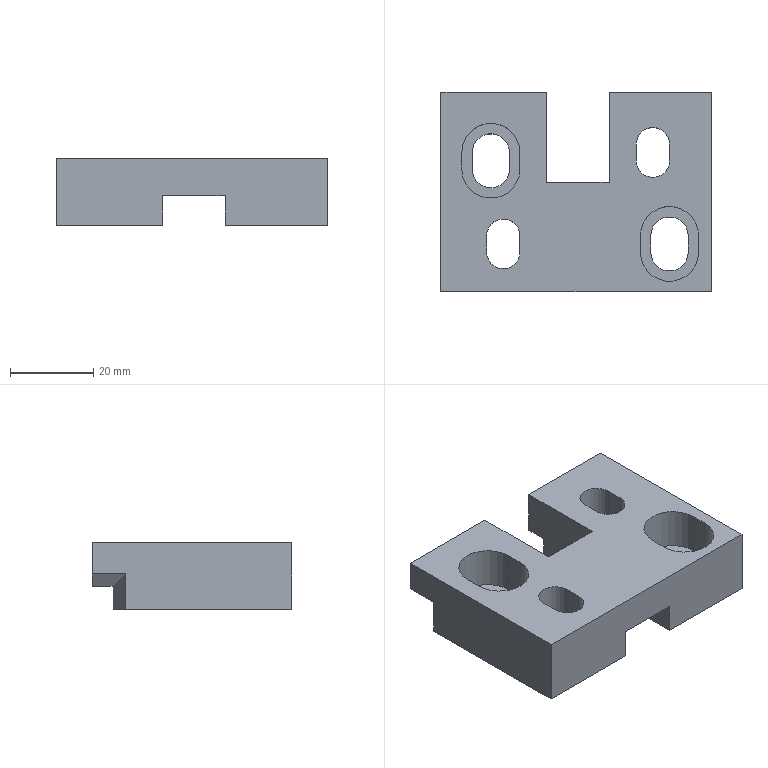Part | STEP file | 1 solid | 46 faces | box 65 x 48 x 16 mm | volume 32002 mm3 | plane 33 | cylinder 13 | commonest cylinder face diameters 8 x4 9 x4 14 x4 5 x1
STEP:
#1=CARTESIAN_POINT('',(-142.451,-110.8,-2.));
#2=VERTEX_POINT('',#1);
#3=CARTESIAN_POINT('',(-142.451,-110.8,4.));
#4=VERTEX_POINT('',#3);
#5=CARTESIAN_POINT('',(-142.451,-110.8,-2.));
#6=DIRECTION('',(0.,0.,1.));
#7=VECTOR('',#6,1.);
#8=LINE('',#5,#7);
#9=EDGE_CURVE('',#2,#4,#8,.T.);
#10=ORIENTED_EDGE('',*,*,#9,.T.);
#11=CARTESIAN_POINT('',(-151.451,-110.8,4.));
#12=VERTEX_POINT('',#11);
#13=CARTESIAN_POINT('',(-146.951,-110.8,4.));
#14=DIRECTION('',(0.,0.,-1.));
#15=DIRECTION('',(-1.,0.,0.));
#16=AXIS2_PLACEMENT_3D('',#13,#14,#15);
#17=CIRCLE('',#16,4.5);
#18=EDGE_CURVE('',#12,#4,#17,.T.);
#19=ORIENTED_EDGE('',*,*,#18,.F.);
#20=CARTESIAN_POINT('',(-151.451,-110.8,-2.));
#21=VERTEX_POINT('',#20);
#22=CARTESIAN_POINT('',(-151.451,-110.8,-2.));
#23=DIRECTION('',(0.,0.,1.));
#24=VECTOR('',#23,1.);
#25=LINE('',#22,#24);
#26=EDGE_CURVE('',#21,#12,#25,.T.);
#27=ORIENTED_EDGE('',*,*,#26,.F.);
#28=CARTESIAN_POINT('',(-146.951,-110.8,-2.));
#29=DIRECTION('',(0.,0.,-1.));
#30=DIRECTION('',(-1.,0.,0.));
#31=AXIS2_PLACEMENT_3D('',#28,#29,#30);
#32=CIRCLE('',#31,4.5);
#33=EDGE_CURVE('',#21,#2,#32,.T.);
#34=ORIENTED_EDGE('',*,*,#33,.T.);
#35=EDGE_LOOP('',(#10,#19,#27,#34));
#36=FACE_OUTER_BOUND('',#35,.T.);
#37=CARTESIAN_POINT('',(-146.951,-110.8,-2.));
#38=DIRECTION('',(0.,0.,1.));
#39=DIRECTION('',(1.,0.,0.));
#40=AXIS2_PLACEMENT_3D('',#37,#38,#39);
#41=CYLINDRICAL_SURFACE('',#40,4.5);
#42=ADVANCED_FACE('',(#36),#41,.F.);
#43=ORIENTED_EDGE('',*,*,#26,.T.);
#44=CARTESIAN_POINT('',(-151.451,-114.8,4.));
#45=VERTEX_POINT('',#44);
#46=CARTESIAN_POINT('',(-151.451,-116.3,4.));
#47=DIRECTION('',(0.,1.,0.));
#48=VECTOR('',#47,1.);
#49=LINE('',#46,#48);
#50=EDGE_CURVE('',#45,#12,#49,.T.);
#51=ORIENTED_EDGE('',*,*,#50,.F.);
#52=CARTESIAN_POINT('',(-151.451,-114.8,-2.));
#53=VERTEX_POINT('',#52);
#54=CARTESIAN_POINT('',(-151.451,-114.8,-2.));
#55=DIRECTION('',(0.,0.,1.));
#56=VECTOR('',#55,1.);
#57=LINE('',#54,#56);
#58=EDGE_CURVE('',#53,#45,#57,.T.);
#59=ORIENTED_EDGE('',*,*,#58,.F.);
#60=CARTESIAN_POINT('',(-151.451,-109.3,-2.));
#61=DIRECTION('',(0.,-1.,0.));
#62=VECTOR('',#61,1.);
#63=LINE('',#60,#62);
#64=EDGE_CURVE('',#21,#53,#63,.T.);
#65=ORIENTED_EDGE('',*,*,#64,.F.);
#66=EDGE_LOOP('',(#43,#51,#59,#65));
#67=FACE_OUTER_BOUND('',#66,.T.);
#68=CARTESIAN_POINT('',(-151.451,-116.3,-2.));
#69=DIRECTION('',(1.,0.,0.));
#70=DIRECTION('',(0.,0.,-1.));
#71=AXIS2_PLACEMENT_3D('',#68,#69,#70);
#72=PLANE('',#71);
#73=ADVANCED_FACE('',(#67),#72,.T.);
#74=ORIENTED_EDGE('',*,*,#58,.T.);
#75=CARTESIAN_POINT('',(-142.451,-114.8,4.));
#76=VERTEX_POINT('',#75);
#77=CARTESIAN_POINT('',(-146.951,-114.8,4.));
#78=DIRECTION('',(0.,0.,-1.));
#79=DIRECTION('',(-1.,0.,0.));
#80=AXIS2_PLACEMENT_3D('',#77,#78,#79);
#81=CIRCLE('',#80,4.5);
#82=EDGE_CURVE('',#76,#45,#81,.T.);
#83=ORIENTED_EDGE('',*,*,#82,.F.);
#84=CARTESIAN_POINT('',(-142.451,-114.8,-2.));
#85=VERTEX_POINT('',#84);
#86=CARTESIAN_POINT('',(-142.451,-114.8,-2.));
#87=DIRECTION('',(0.,0.,1.));
#88=VECTOR('',#87,1.);
#89=LINE('',#86,#88);
#90=EDGE_CURVE('',#85,#76,#89,.T.);
#91=ORIENTED_EDGE('',*,*,#90,.F.);
#92=CARTESIAN_POINT('',(-146.951,-114.8,-2.));
#93=DIRECTION('',(0.,0.,-1.));
#94=DIRECTION('',(-1.,0.,0.));
#95=AXIS2_PLACEMENT_3D('',#92,#93,#94);
#96=CIRCLE('',#95,4.5);
#97=EDGE_CURVE('',#85,#53,#96,.T.);
#98=ORIENTED_EDGE('',*,*,#97,.T.);
#99=EDGE_LOOP('',(#74,#83,#91,#98));
#100=FACE_OUTER_BOUND('',#99,.T.);
#101=CARTESIAN_POINT('',(-146.951,-114.8,-2.));
#102=DIRECTION('',(0.,0.,1.));
#103=DIRECTION('',(1.,0.,0.));
#104=AXIS2_PLACEMENT_3D('',#101,#102,#103);
#105=CYLINDRICAL_SURFACE('',#104,4.5);
#106=ADVANCED_FACE('',(#100),#105,.F.);
#107=ORIENTED_EDGE('',*,*,#90,.T.);
#108=CARTESIAN_POINT('',(-142.451,-109.3,4.));
#109=DIRECTION('',(0.,-1.,0.));
#110=VECTOR('',#109,1.);
#111=LINE('',#108,#110);
#112=EDGE_CURVE('',#4,#76,#111,.T.);
#113=ORIENTED_EDGE('',*,*,#112,.F.);
#114=ORIENTED_EDGE('',*,*,#9,.F.);
#115=CARTESIAN_POINT('',(-142.451,-109.3,-2.));
#116=DIRECTION('',(0.,1.,0.));
#117=VECTOR('',#116,1.);
#118=LINE('',#115,#117);
#119=EDGE_CURVE('',#85,#2,#118,.T.);
#120=ORIENTED_EDGE('',*,*,#119,.F.);
#121=EDGE_LOOP('',(#107,#113,#114,#120));
#122=FACE_OUTER_BOUND('',#121,.T.);
#123=CARTESIAN_POINT('',(-142.451,-109.3,-2.));
#124=DIRECTION('',(-1.,0.,0.));
#125=DIRECTION('',(0.,0.,1.));
#126=AXIS2_PLACEMENT_3D('',#123,#124,#125);
#127=PLANE('',#126);
#128=ADVANCED_FACE('',(#122),#127,.T.);
#129=CARTESIAN_POINT('',(-158.951,-144.3,-2.));
#130=VERTEX_POINT('',#129);
#131=CARTESIAN_POINT('',(-158.951,-144.3,14.));
#132=VERTEX_POINT('',#131);
#133=CARTESIAN_POINT('',(-158.951,-144.3,-2.));
#134=DIRECTION('',(0.,0.,1.));
#135=VECTOR('',#134,1.);
#136=LINE('',#133,#135);
#137=EDGE_CURVE('',#130,#132,#136,.T.);
#138=ORIENTED_EDGE('',*,*,#137,.T.);
#139=CARTESIAN_POINT('',(-158.951,-96.3,14.));
#140=VERTEX_POINT('',#139);
#141=CARTESIAN_POINT('',(-158.951,-94.3,14.));
#142=DIRECTION('',(0.,-1.,0.));
#143=VECTOR('',#142,1.);
#144=LINE('',#141,#143);
#145=EDGE_CURVE('',#140,#132,#144,.T.);
#146=ORIENTED_EDGE('',*,*,#145,.F.);
#147=CARTESIAN_POINT('',(-158.951,-96.3,6.5));
#148=VERTEX_POINT('',#147);
#149=CARTESIAN_POINT('',(-158.951,-96.3,-2.));
#150=DIRECTION('',(0.,0.,-1.));
#151=VECTOR('',#150,1.);
#152=LINE('',#149,#151);
#153=EDGE_CURVE('',#140,#148,#152,.T.);
#154=ORIENTED_EDGE('',*,*,#153,.T.);
#155=CARTESIAN_POINT('',(-158.951,-104.3,6.5));
#156=VERTEX_POINT('',#155);
#157=CARTESIAN_POINT('',(-158.951,-96.3,6.5));
#158=DIRECTION('',(0.,-1.,0.));
#159=VECTOR('',#158,1.);
#160=LINE('',#157,#159);
#161=EDGE_CURVE('',#148,#156,#160,.T.);
#162=ORIENTED_EDGE('',*,*,#161,.T.);
#163=CARTESIAN_POINT('',(-158.951,-104.3,-2.));
#164=VERTEX_POINT('',#163);
#165=CARTESIAN_POINT('',(-158.951,-104.3,-2.));
#166=DIRECTION('',(0.,0.,-1.));
#167=VECTOR('',#166,1.);
#168=LINE('',#165,#167);
#169=EDGE_CURVE('',#156,#164,#168,.T.);
#170=ORIENTED_EDGE('',*,*,#169,.T.);
#171=CARTESIAN_POINT('',(-158.951,-94.3,-2.));
#172=DIRECTION('',(0.,-1.,0.));
#173=VECTOR('',#172,1.);
#174=LINE('',#171,#173);
#175=EDGE_CURVE('',#164,#130,#174,.T.);
#176=ORIENTED_EDGE('',*,*,#175,.T.);
#177=EDGE_LOOP('',(#138,#146,#154,#162,#170,#176));
#178=FACE_OUTER_BOUND('',#177,.T.);
#179=CARTESIAN_POINT('',(-158.951,-94.3,-2.));
#180=DIRECTION('',(-1.,0.,0.));
#181=DIRECTION('',(0.,0.,1.));
#182=AXIS2_PLACEMENT_3D('',#179,#180,#181);
#183=PLANE('',#182);
#184=ADVANCED_FACE('',(#178),#183,.T.);
#185=CARTESIAN_POINT('',(-133.5,-101.3,3.5));
#186=VERTEX_POINT('',#185);
#187=CARTESIAN_POINT('',(-133.5,-101.3,-2.));
#188=VERTEX_POINT('',#187);
#189=CARTESIAN_POINT('',(-133.5,-101.3,7.75));
#190=DIRECTION('',(0.,0.,-1.));
#191=VECTOR('',#190,1.);
#192=LINE('',#189,#191);
#193=EDGE_CURVE('',#186,#188,#192,.T.);
#194=ORIENTED_EDGE('',*,*,#193,.F.);
#195=CARTESIAN_POINT('',(-133.5,-96.3,3.5));
#196=VERTEX_POINT('',#195);
#197=CARTESIAN_POINT('',(-133.5,-81.,3.5));
#198=DIRECTION('',(0.,1.,0.));
#199=VECTOR('',#198,1.);
#200=LINE('',#197,#199);
#201=EDGE_CURVE('',#186,#196,#200,.T.);
#202=ORIENTED_EDGE('',*,*,#201,.T.);
#203=CARTESIAN_POINT('',(-133.5,-96.3,14.));
#204=VERTEX_POINT('',#203);
#205=CARTESIAN_POINT('',(-133.5,-96.3,7.75));
#206=DIRECTION('',(0.,0.,-1.));
#207=VECTOR('',#206,1.);
#208=LINE('',#205,#207);
#209=EDGE_CURVE('',#204,#196,#208,.T.);
#210=ORIENTED_EDGE('',*,*,#209,.F.);
#211=CARTESIAN_POINT('',(-133.5,-118.,14.));
#212=VERTEX_POINT('',#211);
#213=CARTESIAN_POINT('',(-133.5,-109.3,14.));
#214=DIRECTION('',(0.,-1.,0.));
#215=VECTOR('',#214,1.);
#216=LINE('',#213,#215);
#217=EDGE_CURVE('',#204,#212,#216,.T.);
#218=ORIENTED_EDGE('',*,*,#217,.T.);
#219=CARTESIAN_POINT('',(-133.5,-118.,5.1));
#220=VERTEX_POINT('',#219);
#221=CARTESIAN_POINT('',(-133.5,-118.,-195.));
#222=DIRECTION('',(0.,0.,1.));
#223=VECTOR('',#222,1.);
#224=LINE('',#221,#223);
#225=EDGE_CURVE('',#220,#212,#224,.T.);
#226=ORIENTED_EDGE('',*,*,#225,.F.);
#227=CARTESIAN_POINT('',(-133.5,-144.3,5.1));
#228=VERTEX_POINT('',#227);
#229=CARTESIAN_POINT('',(-133.5,-79.,5.1));
#230=DIRECTION('',(0.,-1.,0.));
#231=VECTOR('',#230,1.);
#232=LINE('',#229,#231);
#233=EDGE_CURVE('',#220,#228,#232,.T.);
#234=ORIENTED_EDGE('',*,*,#233,.T.);
#235=CARTESIAN_POINT('',(-133.5,-144.3,-2.));
#236=VERTEX_POINT('',#235);
#237=CARTESIAN_POINT('',(-133.5,-144.3,-2.));
#238=DIRECTION('',(0.,0.,1.));
#239=VECTOR('',#238,1.);
#240=LINE('',#237,#239);
#241=EDGE_CURVE('',#236,#228,#240,.T.);
#242=ORIENTED_EDGE('',*,*,#241,.F.);
#243=CARTESIAN_POINT('',(-133.5,-109.3,-2.));
#244=DIRECTION('',(0.,-1.,0.));
#245=VECTOR('',#244,1.);
#246=LINE('',#243,#245);
#247=EDGE_CURVE('',#188,#236,#246,.T.);
#248=ORIENTED_EDGE('',*,*,#247,.F.);
#249=EDGE_LOOP('',(#194,#202,#210,#218,#226,#234,#242,#248));
#250=FACE_OUTER_BOUND('',#249,.T.);
#251=CARTESIAN_POINT('',(-133.5,-79.,-195.));
#252=DIRECTION('',(1.,0.,0.));
#253=DIRECTION('',(0.,0.,-1.));
#254=AXIS2_PLACEMENT_3D('',#251,#252,#253);
#255=PLANE('',#254);
#256=ADVANCED_FACE('',(#250),#255,.T.);
#257=CARTESIAN_POINT('',(-148.951,-101.3,3.5));
#258=VERTEX_POINT('',#257);
#259=CARTESIAN_POINT('',(-130.951,-101.3,3.5));
#260=DIRECTION('',(1.,0.,0.));
#261=VECTOR('',#260,1.);
#262=LINE('',#259,#261);
#263=EDGE_CURVE('',#258,#186,#262,.T.);
#264=ORIENTED_EDGE('',*,*,#263,.T.);
#265=ORIENTED_EDGE('',*,*,#193,.T.);
#266=CARTESIAN_POINT('',(-148.951,-101.3,-2.));
#267=VERTEX_POINT('',#266);
#268=CARTESIAN_POINT('',(-130.951,-101.3,-2.));
#269=DIRECTION('',(1.,0.,0.));
#270=VECTOR('',#269,1.);
#271=LINE('',#268,#270);
#272=EDGE_CURVE('',#267,#188,#271,.T.);
#273=ORIENTED_EDGE('',*,*,#272,.F.);
#274=CARTESIAN_POINT('',(-148.951,-101.3,-18.));
#275=DIRECTION('',(0.,0.,1.));
#276=VECTOR('',#275,1.);
#277=LINE('',#274,#276);
#278=EDGE_CURVE('',#267,#258,#277,.T.);
#279=ORIENTED_EDGE('',*,*,#278,.T.);
#280=EDGE_LOOP('',(#264,#265,#273,#279));
#281=FACE_OUTER_BOUND('',#280,.T.);
#282=CARTESIAN_POINT('',(-65.951,-101.3,-18.));
#283=DIRECTION('',(0.,1.,0.));
#284=DIRECTION('',(0.,0.,1.));
#285=AXIS2_PLACEMENT_3D('',#282,#283,#284);
#286=PLANE('',#285);
#287=ADVANCED_FACE('',(#281),#286,.T.);
#288=ORIENTED_EDGE('',*,*,#169,.F.);
#289=CARTESIAN_POINT('',(-156.918,-103.69,5.89));
#290=DIRECTION('',(-0.9206,-0.2762,0.2762));
#291=VECTOR('',#290,1.);
#292=LINE('',#289,#291);
#293=EDGE_CURVE('',#258,#156,#292,.T.);
#294=ORIENTED_EDGE('',*,*,#293,.F.);
#295=ORIENTED_EDGE('',*,*,#278,.F.);
#296=CARTESIAN_POINT('',(-87.484,-82.86,-2.));
#297=DIRECTION('',(0.9578,0.2873,0.));
#298=VECTOR('',#297,1.);
#299=LINE('',#296,#298);
#300=EDGE_CURVE('',#164,#267,#299,.T.);
#301=ORIENTED_EDGE('',*,*,#300,.F.);
#302=EDGE_LOOP('',(#288,#294,#295,#301));
#303=FACE_OUTER_BOUND('',#302,.T.);
#304=CARTESIAN_POINT('',(-148.951,-101.3,-18.));
#305=DIRECTION('',(0.2873,-0.9578,0.));
#306=DIRECTION('',(0.,0.,1.));
#307=AXIS2_PLACEMENT_3D('',#304,#305,#306);
#308=PLANE('',#307);
#309=ADVANCED_FACE('',(#303),#308,.F.);
#310=ORIENTED_EDGE('',*,*,#241,.T.);
#311=CARTESIAN_POINT('',(-118.5,-144.3,5.1));
#312=VERTEX_POINT('',#311);
#313=CARTESIAN_POINT('',(-170.951,-144.3,5.1));
#314=DIRECTION('',(-1.,0.,0.));
#315=VECTOR('',#314,1.);
#316=LINE('',#313,#315);
#317=EDGE_CURVE('',#312,#228,#316,.T.);
#318=ORIENTED_EDGE('',*,*,#317,.F.);
#319=CARTESIAN_POINT('',(-118.5,-144.3,-2.));
#320=VERTEX_POINT('',#319);
#321=CARTESIAN_POINT('',(-118.5,-144.3,-2.));
#322=DIRECTION('',(0.,0.,1.));
#323=VECTOR('',#322,1.);
#324=LINE('',#321,#323);
#325=EDGE_CURVE('',#320,#312,#324,.T.);
#326=ORIENTED_EDGE('',*,*,#325,.F.);
#327=CARTESIAN_POINT('',(-93.951,-144.3,-2.));
#328=VERTEX_POINT('',#327);
#329=CARTESIAN_POINT('',(-170.951,-144.3,-2.));
#330=DIRECTION('',(1.,0.,0.));
#331=VECTOR('',#330,1.);
#332=LINE('',#329,#331);
#333=EDGE_CURVE('',#320,#328,#332,.T.);
#334=ORIENTED_EDGE('',*,*,#333,.T.);
#335=CARTESIAN_POINT('',(-93.951,-144.3,14.));
#336=VERTEX_POINT('',#335);
#337=CARTESIAN_POINT('',(-93.951,-144.3,-2.));
#338=DIRECTION('',(0.,0.,-1.));
#339=VECTOR('',#338,1.);
#340=LINE('',#337,#339);
#341=EDGE_CURVE('',#336,#328,#340,.T.);
#342=ORIENTED_EDGE('',*,*,#341,.F.);
#343=CARTESIAN_POINT('',(-170.951,-144.3,14.));
#344=DIRECTION('',(1.,0.,0.));
#345=VECTOR('',#344,1.);
#346=LINE('',#343,#345);
#347=EDGE_CURVE('',#132,#336,#346,.T.);
#348=ORIENTED_EDGE('',*,*,#347,.F.);
#349=ORIENTED_EDGE('',*,*,#137,.F.);
#350=CARTESIAN_POINT('',(-170.951,-144.3,-2.));
#351=DIRECTION('',(1.,0.,0.));
#352=VECTOR('',#351,1.);
#353=LINE('',#350,#352);
#354=EDGE_CURVE('',#130,#236,#353,.T.);
#355=ORIENTED_EDGE('',*,*,#354,.T.);
#356=EDGE_LOOP('',(#310,#318,#326,#334,#342,#348,#349,#355));
#357=FACE_OUTER_BOUND('',#356,.T.);
#358=CARTESIAN_POINT('',(-170.951,-144.3,-2.));
#359=DIRECTION('',(0.,-1.,0.));
#360=DIRECTION('',(0.,0.,-1.));
#361=AXIS2_PLACEMENT_3D('',#358,#359,#360);
#362=PLANE('',#361);
#363=ADVANCED_FACE('',(#357),#362,.T.);
#364=ORIENTED_EDGE('',*,*,#354,.F.);
#365=ORIENTED_EDGE('',*,*,#175,.F.);
#366=ORIENTED_EDGE('',*,*,#300,.T.);
#367=ORIENTED_EDGE('',*,*,#272,.T.);
#368=ORIENTED_EDGE('',*,*,#247,.T.);
#369=EDGE_LOOP('',(#364,#365,#366,#367,#368));
#370=FACE_BOUND('',#369,.T.);
#371=CARTESIAN_POINT('',(-139.951,-130.8,-2.));
#372=VERTEX_POINT('',#371);
#373=CARTESIAN_POINT('',(-139.951,-134.8,-2.));
#374=VERTEX_POINT('',#373);
#375=CARTESIAN_POINT('',(-139.951,-129.3,-2.));
#376=DIRECTION('',(0.,-1.,0.));
#377=VECTOR('',#376,1.);
#378=LINE('',#375,#377);
#379=EDGE_CURVE('',#372,#374,#378,.T.);
#380=ORIENTED_EDGE('',*,*,#379,.F.);
#381=CARTESIAN_POINT('',(-147.951,-130.8,-2.));
#382=VERTEX_POINT('',#381);
#383=CARTESIAN_POINT('',(-143.951,-130.8,-2.));
#384=DIRECTION('',(0.,0.,-1.));
#385=DIRECTION('',(-1.,0.,0.));
#386=AXIS2_PLACEMENT_3D('',#383,#384,#385);
#387=CIRCLE('',#386,4.);
#388=EDGE_CURVE('',#382,#372,#387,.T.);
#389=ORIENTED_EDGE('',*,*,#388,.F.);
#390=CARTESIAN_POINT('',(-147.951,-134.8,-2.));
#391=VERTEX_POINT('',#390);
#392=CARTESIAN_POINT('',(-147.951,-129.3,-2.));
#393=DIRECTION('',(0.,1.,0.));
#394=VECTOR('',#393,1.);
#395=LINE('',#392,#394);
#396=EDGE_CURVE('',#391,#382,#395,.T.);
#397=ORIENTED_EDGE('',*,*,#396,.F.);
#398=CARTESIAN_POINT('',(-143.951,-134.8,-2.));
#399=DIRECTION('',(0.,0.,-1.));
#400=DIRECTION('',(-1.,0.,0.));
#401=AXIS2_PLACEMENT_3D('',#398,#399,#400);
#402=CIRCLE('',#401,4.);
#403=EDGE_CURVE('',#374,#391,#402,.T.);
#404=ORIENTED_EDGE('',*,*,#403,.F.);
#405=EDGE_LOOP('',(#380,#389,#397,#404));
#406=FACE_BOUND('',#405,.T.);
#407=ORIENTED_EDGE('',*,*,#33,.F.);
#408=ORIENTED_EDGE('',*,*,#64,.T.);
#409=ORIENTED_EDGE('',*,*,#97,.F.);
#410=ORIENTED_EDGE('',*,*,#119,.T.);
#411=EDGE_LOOP('',(#407,#408,#409,#410));
#412=FACE_BOUND('',#411,.T.);
#413=CARTESIAN_POINT('',(-145.951,-109.3,-2.));
#414=DIRECTION('',(0.,0.,-1.));
#415=DIRECTION('',(-1.,0.,0.));
#416=AXIS2_PLACEMENT_3D('',#413,#414,#415);
#417=PLANE('',#416);
#418=ADVANCED_FACE('',(#370,#406,#412),#417,.T.);
#419=CARTESIAN_POINT('',(-147.951,-130.8,14.));
#420=VERTEX_POINT('',#419);
#421=CARTESIAN_POINT('',(-147.951,-130.8,-2.));
#422=DIRECTION('',(0.,0.,1.));
#423=VECTOR('',#422,1.);
#424=LINE('',#421,#423);
#425=EDGE_CURVE('',#382,#420,#424,.T.);
#426=ORIENTED_EDGE('',*,*,#425,.T.);
#427=CARTESIAN_POINT('',(-147.951,-134.8,14.));
#428=VERTEX_POINT('',#427);
#429=CARTESIAN_POINT('',(-147.951,-129.3,14.));
#430=DIRECTION('',(0.,1.,0.));
#431=VECTOR('',#430,1.);
#432=LINE('',#429,#431);
#433=EDGE_CURVE('',#428,#420,#432,.T.);
#434=ORIENTED_EDGE('',*,*,#433,.F.);
#435=CARTESIAN_POINT('',(-147.951,-134.8,-2.));
#436=DIRECTION('',(0.,0.,1.));
#437=VECTOR('',#436,1.);
#438=LINE('',#435,#437);
#439=EDGE_CURVE('',#391,#428,#438,.T.);
#440=ORIENTED_EDGE('',*,*,#439,.F.);
#441=ORIENTED_EDGE('',*,*,#396,.T.);
#442=EDGE_LOOP('',(#426,#434,#440,#441));
#443=FACE_OUTER_BOUND('',#442,.T.);
#444=CARTESIAN_POINT('',(-147.951,-129.3,-2.));
#445=DIRECTION('',(-1.,0.,0.));
#446=DIRECTION('',(0.,0.,1.));
#447=AXIS2_PLACEMENT_3D('',#444,#445,#446);
#448=PLANE('',#447);
#449=ADVANCED_FACE('',(#443),#448,.F.);
#450=CARTESIAN_POINT('',(-139.951,-130.8,14.));
#451=VERTEX_POINT('',#450);
#452=CARTESIAN_POINT('',(-139.951,-130.8,-2.));
#453=DIRECTION('',(0.,0.,1.));
#454=VECTOR('',#453,1.);
#455=LINE('',#452,#454);
#456=EDGE_CURVE('',#372,#451,#455,.T.);
#457=ORIENTED_EDGE('',*,*,#456,.T.);
#458=CARTESIAN_POINT('',(-143.951,-130.8,14.));
#459=DIRECTION('',(0.,0.,-1.));
#460=DIRECTION('',(-1.,0.,0.));
#461=AXIS2_PLACEMENT_3D('',#458,#459,#460);
#462=CIRCLE('',#461,4.);
#463=EDGE_CURVE('',#420,#451,#462,.T.);
#464=ORIENTED_EDGE('',*,*,#463,.F.);
#465=ORIENTED_EDGE('',*,*,#425,.F.);
#466=ORIENTED_EDGE('',*,*,#388,.T.);
#467=EDGE_LOOP('',(#457,#464,#465,#466));
#468=FACE_OUTER_BOUND('',#467,.T.);
#469=CARTESIAN_POINT('',(-143.951,-130.8,-2.));
#470=DIRECTION('',(0.,0.,1.));
#471=DIRECTION('',(1.,0.,0.));
#472=AXIS2_PLACEMENT_3D('',#469,#470,#471);
#473=CYLINDRICAL_SURFACE('',#472,4.);
#474=ADVANCED_FACE('',(#468),#473,.F.);
#475=CARTESIAN_POINT('',(-139.951,-134.8,14.));
#476=VERTEX_POINT('',#475);
#477=CARTESIAN_POINT('',(-139.951,-134.8,-2.));
#478=DIRECTION('',(0.,0.,1.));
#479=VECTOR('',#478,1.);
#480=LINE('',#477,#479);
#481=EDGE_CURVE('',#374,#476,#480,.T.);
#482=ORIENTED_EDGE('',*,*,#481,.T.);
#483=CARTESIAN_POINT('',(-139.951,-129.3,14.));
#484=DIRECTION('',(0.,-1.,0.));
#485=VECTOR('',#484,1.);
#486=LINE('',#483,#485);
#487=EDGE_CURVE('',#451,#476,#486,.T.);
#488=ORIENTED_EDGE('',*,*,#487,.F.);
#489=ORIENTED_EDGE('',*,*,#456,.F.);
#490=ORIENTED_EDGE('',*,*,#379,.T.);
#491=EDGE_LOOP('',(#482,#488,#489,#490));
#492=FACE_OUTER_BOUND('',#491,.T.);
#493=CARTESIAN_POINT('',(-139.951,-136.3,-2.));
#494=DIRECTION('',(1.,0.,0.));
#495=DIRECTION('',(0.,0.,-1.));
#496=AXIS2_PLACEMENT_3D('',#493,#494,#495);
#497=PLANE('',#496);
#498=ADVANCED_FACE('',(#492),#497,.F.);
#499=ORIENTED_EDGE('',*,*,#439,.T.);
#500=CARTESIAN_POINT('',(-143.951,-134.8,14.));
#501=DIRECTION('',(0.,0.,-1.));
#502=DIRECTION('',(-1.,0.,0.));
#503=AXIS2_PLACEMENT_3D('',#500,#501,#502);
#504=CIRCLE('',#503,4.);
#505=EDGE_CURVE('',#476,#428,#504,.T.);
#506=ORIENTED_EDGE('',*,*,#505,.F.);
#507=ORIENTED_EDGE('',*,*,#481,.F.);
#508=ORIENTED_EDGE('',*,*,#403,.T.);
#509=EDGE_LOOP('',(#499,#506,#507,#508));
#510=FACE_OUTER_BOUND('',#509,.T.);
#511=CARTESIAN_POINT('',(-143.951,-134.8,-2.));
#512=DIRECTION('',(0.,0.,1.));
#513=DIRECTION('',(1.,0.,0.));
#514=AXIS2_PLACEMENT_3D('',#511,#512,#513);
#515=CYLINDRICAL_SURFACE('',#514,4.);
#516=ADVANCED_FACE('',(#510),#515,.F.);
#517=ORIENTED_EDGE('',*,*,#263,.F.);
#518=CARTESIAN_POINT('',(-148.951,-96.3,3.5));
#519=VERTEX_POINT('',#518);
#520=CARTESIAN_POINT('',(-148.951,-111.3,3.5));
#521=DIRECTION('',(0.,1.,0.));
#522=VECTOR('',#521,1.);
#523=LINE('',#520,#522);
#524=EDGE_CURVE('',#258,#519,#523,.T.);
#525=ORIENTED_EDGE('',*,*,#524,.T.);
#526=CARTESIAN_POINT('',(-166.,-96.3,3.5));
#527=DIRECTION('',(-1.,0.,0.));
#528=VECTOR('',#527,1.);
#529=LINE('',#526,#528);
#530=EDGE_CURVE('',#196,#519,#529,.T.);
#531=ORIENTED_EDGE('',*,*,#530,.F.);
#532=ORIENTED_EDGE('',*,*,#201,.F.);
#533=EDGE_LOOP('',(#517,#525,#531,#532));
#534=FACE_OUTER_BOUND('',#533,.T.);
#535=CARTESIAN_POINT('',(-130.951,-111.3,3.5));
#536=DIRECTION('',(0.,0.,-1.));
#537=DIRECTION('',(-1.,0.,0.));
#538=AXIS2_PLACEMENT_3D('',#535,#536,#537);
#539=PLANE('',#538);
#540=ADVANCED_FACE('',(#534),#539,.T.);
#541=CARTESIAN_POINT('',(-110.951,-130.8,14.));
#542=VERTEX_POINT('',#541);
#543=CARTESIAN_POINT('',(-110.951,-134.8,14.));
#544=VERTEX_POINT('',#543);
#545=CARTESIAN_POINT('',(-110.951,-129.3,14.));
#546=DIRECTION('',(0.,-1.,0.));
#547=VECTOR('',#546,1.);
#548=LINE('',#545,#547);
#549=EDGE_CURVE('',#542,#544,#548,.T.);
#550=ORIENTED_EDGE('',*,*,#549,.F.);
#551=CARTESIAN_POINT('',(-96.951,-130.8,14.));
#552=VERTEX_POINT('',#551);
#553=CARTESIAN_POINT('',(-103.951,-130.8,14.));
#554=DIRECTION('',(0.,0.,-1.));
#555=DIRECTION('',(-1.,0.,0.));
#556=AXIS2_PLACEMENT_3D('',#553,#554,#555);
#557=CIRCLE('',#556,7.);
#558=EDGE_CURVE('',#542,#552,#557,.T.);
#559=ORIENTED_EDGE('',*,*,#558,.T.);
#560=CARTESIAN_POINT('',(-96.951,-134.8,14.));
#561=VERTEX_POINT('',#560);
#562=CARTESIAN_POINT('',(-96.951,-129.3,14.));
#563=DIRECTION('',(0.,1.,0.));
#564=VECTOR('',#563,1.);
#565=LINE('',#562,#564);
#566=EDGE_CURVE('',#561,#552,#565,.T.);
#567=ORIENTED_EDGE('',*,*,#566,.F.);
#568=CARTESIAN_POINT('',(-103.951,-134.8,14.));
#569=DIRECTION('',(0.,0.,-1.));
#570=DIRECTION('',(-1.,0.,0.));
#571=AXIS2_PLACEMENT_3D('',#568,#569,#570);
#572=CIRCLE('',#571,7.);
#573=EDGE_CURVE('',#561,#544,#572,.T.);
#574=ORIENTED_EDGE('',*,*,#573,.T.);
#575=EDGE_LOOP('',(#550,#559,#567,#574));
#576=FACE_BOUND('',#575,.T.);
#577=CARTESIAN_POINT('',(-111.951,-112.8,14.));
#578=VERTEX_POINT('',#577);
#579=CARTESIAN_POINT('',(-111.951,-108.8,14.));
#580=VERTEX_POINT('',#579);
#581=CARTESIAN_POINT('',(-111.951,-107.3,14.));
#582=DIRECTION('',(0.,1.,0.));
#583=VECTOR('',#582,1.);
#584=LINE('',#581,#583);
#585=EDGE_CURVE('',#578,#580,#584,.T.);
#586=ORIENTED_EDGE('',*,*,#585,.T.);
#587=CARTESIAN_POINT('',(-103.951,-108.8,14.));
#588=VERTEX_POINT('',#587);
#589=CARTESIAN_POINT('',(-107.951,-108.8,14.));
#590=DIRECTION('',(0.,0.,-1.));
#591=DIRECTION('',(-1.,0.,0.));
#592=AXIS2_PLACEMENT_3D('',#589,#590,#591);
#593=CIRCLE('',#592,4.);
#594=EDGE_CURVE('',#580,#588,#593,.T.);
#595=ORIENTED_EDGE('',*,*,#594,.T.);
#596=CARTESIAN_POINT('',(-103.951,-112.8,14.));
#597=VERTEX_POINT('',#596);
#598=CARTESIAN_POINT('',(-103.951,-107.3,14.));
#599=DIRECTION('',(0.,-1.,0.));
#600=VECTOR('',#599,1.);
#601=LINE('',#598,#600);
#602=EDGE_CURVE('',#588,#597,#601,.T.);
#603=ORIENTED_EDGE('',*,*,#602,.T.);
#604=CARTESIAN_POINT('',(-107.951,-112.8,14.));
#605=DIRECTION('',(0.,0.,-1.));
#606=DIRECTION('',(-1.,0.,0.));
#607=AXIS2_PLACEMENT_3D('',#604,#605,#606);
#608=CIRCLE('',#607,4.);
#609=EDGE_CURVE('',#597,#578,#608,.T.);
#610=ORIENTED_EDGE('',*,*,#609,.T.);
#611=EDGE_LOOP('',(#586,#595,#603,#610));
#612=FACE_BOUND('',#611,.T.);
#613=ORIENTED_EDGE('',*,*,#433,.T.);
#614=ORIENTED_EDGE('',*,*,#463,.T.);
#615=ORIENTED_EDGE('',*,*,#487,.T.);
#616=ORIENTED_EDGE('',*,*,#505,.T.);
#617=EDGE_LOOP('',(#613,#614,#615,#616));
#618=FACE_BOUND('',#617,.T.);
#619=CARTESIAN_POINT('',(-153.951,-110.8,14.));
#620=VERTEX_POINT('',#619);
#621=CARTESIAN_POINT('',(-153.951,-114.8,14.));
#622=VERTEX_POINT('',#621);
#623=CARTESIAN_POINT('',(-153.951,-109.3,14.));
#624=DIRECTION('',(0.,-1.,0.));
#625=VECTOR('',#624,1.);
#626=LINE('',#623,#625);
#627=EDGE_CURVE('',#620,#622,#626,.T.);
#628=ORIENTED_EDGE('',*,*,#627,.F.);
#629=CARTESIAN_POINT('',(-139.951,-110.8,14.));
#630=VERTEX_POINT('',#629);
#631=CARTESIAN_POINT('',(-146.951,-110.8,14.));
#632=DIRECTION('',(0.,0.,-1.));
#633=DIRECTION('',(-1.,0.,0.));
#634=AXIS2_PLACEMENT_3D('',#631,#632,#633);
#635=CIRCLE('',#634,7.);
#636=EDGE_CURVE('',#620,#630,#635,.T.);
#637=ORIENTED_EDGE('',*,*,#636,.T.);
#638=CARTESIAN_POINT('',(-139.951,-114.8,14.));
#639=VERTEX_POINT('',#638);
#640=CARTESIAN_POINT('',(-139.951,-109.3,14.));
#641=DIRECTION('',(0.,1.,0.));
#642=VECTOR('',#641,1.);
#643=LINE('',#640,#642);
#644=EDGE_CURVE('',#639,#630,#643,.T.);
#645=ORIENTED_EDGE('',*,*,#644,.F.);
#646=CARTESIAN_POINT('',(-146.951,-114.8,14.));
#647=DIRECTION('',(0.,0.,-1.));
#648=DIRECTION('',(-1.,0.,0.));
#649=AXIS2_PLACEMENT_3D('',#646,#647,#648);
#650=CIRCLE('',#649,7.);
#651=EDGE_CURVE('',#639,#622,#650,.T.);
#652=ORIENTED_EDGE('',*,*,#651,.T.);
#653=EDGE_LOOP('',(#628,#637,#645,#652));
#654=FACE_BOUND('',#653,.T.);
#655=CARTESIAN_POINT('',(-145.951,-96.3,14.));
#656=DIRECTION('',(-1.,0.,0.));
#657=VECTOR('',#656,1.);
#658=LINE('',#655,#657);
#659=EDGE_CURVE('',#204,#140,#658,.T.);
#660=ORIENTED_EDGE('',*,*,#659,.T.);
#661=ORIENTED_EDGE('',*,*,#145,.T.);
#662=ORIENTED_EDGE('',*,*,#347,.T.);
#663=CARTESIAN_POINT('',(-93.951,-96.3,14.));
#664=VERTEX_POINT('',#663);
#665=CARTESIAN_POINT('',(-93.951,-109.3,14.));
#666=DIRECTION('',(0.,1.,0.));
#667=VECTOR('',#666,1.);
#668=LINE('',#665,#667);
#669=EDGE_CURVE('',#336,#664,#668,.T.);
#670=ORIENTED_EDGE('',*,*,#669,.T.);
#671=CARTESIAN_POINT('',(-118.5,-96.3,14.));
#672=VERTEX_POINT('',#671);
#673=CARTESIAN_POINT('',(-70.951,-96.3,14.));
#674=DIRECTION('',(-1.,0.,0.));
#675=VECTOR('',#674,1.);
#676=LINE('',#673,#675);
#677=EDGE_CURVE('',#664,#672,#676,.T.);
#678=ORIENTED_EDGE('',*,*,#677,.T.);
#679=CARTESIAN_POINT('',(-118.5,-118.,14.));
#680=VERTEX_POINT('',#679);
#681=CARTESIAN_POINT('',(-118.5,-109.3,14.));
#682=DIRECTION('',(0.,-1.,0.));
#683=VECTOR('',#682,1.);
#684=LINE('',#681,#683);
#685=EDGE_CURVE('',#672,#680,#684,.T.);
#686=ORIENTED_EDGE('',*,*,#685,.T.);
#687=CARTESIAN_POINT('',(-145.951,-118.,14.));
#688=DIRECTION('',(1.,0.,0.));
#689=VECTOR('',#688,1.);
#690=LINE('',#687,#689);
#691=EDGE_CURVE('',#212,#680,#690,.T.);
#692=ORIENTED_EDGE('',*,*,#691,.F.);
#693=ORIENTED_EDGE('',*,*,#217,.F.);
#694=EDGE_LOOP('',(#660,#661,#662,#670,#678,#686,#692,#693));
#695=FACE_BOUND('',#694,.T.);
#696=CARTESIAN_POINT('',(-145.951,-109.3,14.));
#697=DIRECTION('',(0.,0.,-1.));
#698=DIRECTION('',(-1.,0.,0.));
#699=AXIS2_PLACEMENT_3D('',#696,#697,#698);
#700=PLANE('',#699);
#701=ADVANCED_FACE('',(#576,#612,#618,#654,#695),#700,.F.);
#702=CARTESIAN_POINT('',(-118.5,-96.3,3.5));
#703=VERTEX_POINT('',#702);
#704=CARTESIAN_POINT('',(-118.5,-101.3,3.5));
#705=VERTEX_POINT('',#704);
#706=CARTESIAN_POINT('',(-118.5,-111.3,3.5));
#707=DIRECTION('',(0.,-1.,0.));
#708=VECTOR('',#707,1.);
#709=LINE('',#706,#708);
#710=EDGE_CURVE('',#703,#705,#709,.T.);
#711=ORIENTED_EDGE('',*,*,#710,.T.);
#712=CARTESIAN_POINT('',(-118.5,-101.3,-2.));
#713=VERTEX_POINT('',#712);
#714=CARTESIAN_POINT('',(-118.5,-101.3,-18.));
#715=DIRECTION('',(0.,0.,-1.));
#716=VECTOR('',#715,1.);
#717=LINE('',#714,#716);
#718=EDGE_CURVE('',#705,#713,#717,.T.);
#719=ORIENTED_EDGE('',*,*,#718,.T.);
#720=CARTESIAN_POINT('',(-118.5,-109.3,-2.));
#721=DIRECTION('',(0.,-1.,0.));
#722=VECTOR('',#721,1.);
#723=LINE('',#720,#722);
#724=EDGE_CURVE('',#713,#320,#723,.T.);
#725=ORIENTED_EDGE('',*,*,#724,.T.);
#726=ORIENTED_EDGE('',*,*,#325,.T.);
#727=CARTESIAN_POINT('',(-118.5,-118.,5.1));
#728=VERTEX_POINT('',#727);
#729=CARTESIAN_POINT('',(-118.5,-79.,5.1));
#730=DIRECTION('',(0.,-1.,0.));
#731=VECTOR('',#730,1.);
#732=LINE('',#729,#731);
#733=EDGE_CURVE('',#728,#312,#732,.T.);
#734=ORIENTED_EDGE('',*,*,#733,.F.);
#735=CARTESIAN_POINT('',(-118.5,-118.,9.));
#736=DIRECTION('',(0.,0.,-1.));
#737=VECTOR('',#736,1.);
#738=LINE('',#735,#737);
#739=EDGE_CURVE('',#680,#728,#738,.T.);
#740=ORIENTED_EDGE('',*,*,#739,.F.);
#741=ORIENTED_EDGE('',*,*,#685,.F.);
#742=CARTESIAN_POINT('',(-118.5,-96.3,-195.));
#743=DIRECTION('',(0.,0.,1.));
#744=VECTOR('',#743,1.);
#745=LINE('',#742,#744);
#746=EDGE_CURVE('',#703,#672,#745,.T.);
#747=ORIENTED_EDGE('',*,*,#746,.F.);
#748=EDGE_LOOP('',(#711,#719,#725,#726,#734,#740,#741,#747));
#749=FACE_OUTER_BOUND('',#748,.T.);
#750=CARTESIAN_POINT('',(-118.5,-79.,-195.));
#751=DIRECTION('',(1.,0.,0.));
#752=DIRECTION('',(0.,0.,-1.));
#753=AXIS2_PLACEMENT_3D('',#750,#751,#752);
#754=PLANE('',#753);
#755=ADVANCED_FACE('',(#749),#754,.F.);
#756=ORIENTED_EDGE('',*,*,#659,.F.);
#757=ORIENTED_EDGE('',*,*,#209,.T.);
#758=ORIENTED_EDGE('',*,*,#530,.T.);
#759=CARTESIAN_POINT('',(-14.961,-96.3,-36.697));
#760=DIRECTION('',(-0.9578,0.,0.2873));
#761=VECTOR('',#760,1.);
#762=LINE('',#759,#761);
#763=EDGE_CURVE('',#519,#148,#762,.T.);
#764=ORIENTED_EDGE('',*,*,#763,.T.);
#765=ORIENTED_EDGE('',*,*,#153,.F.);
#766=EDGE_LOOP('',(#756,#757,#758,#764,#765));
#767=FACE_OUTER_BOUND('',#766,.T.);
#768=CARTESIAN_POINT('',(-166.,-96.3,7.75));
#769=DIRECTION('',(0.,1.,0.));
#770=DIRECTION('',(0.,0.,1.));
#771=AXIS2_PLACEMENT_3D('',#768,#769,#770);
#772=PLANE('',#771);
#773=ADVANCED_FACE('',(#767),#772,.T.);
#774=CARTESIAN_POINT('',(-103.951,-112.8,-2.));
#775=VERTEX_POINT('',#774);
#776=CARTESIAN_POINT('',(-103.951,-112.8,-2.));
#777=DIRECTION('',(0.,0.,1.));
#778=VECTOR('',#777,1.);
#779=LINE('',#776,#778);
#780=EDGE_CURVE('',#775,#597,#779,.T.);
#781=ORIENTED_EDGE('',*,*,#780,.F.);
#782=CARTESIAN_POINT('',(-111.951,-112.8,-2.));
#783=VERTEX_POINT('',#782);
#784=CARTESIAN_POINT('',(-107.951,-112.8,-2.));
#785=DIRECTION('',(0.,0.,-1.));
#786=DIRECTION('',(-1.,0.,0.));
#787=AXIS2_PLACEMENT_3D('',#784,#785,#786);
#788=CIRCLE('',#787,4.);
#789=EDGE_CURVE('',#775,#783,#788,.T.);
#790=ORIENTED_EDGE('',*,*,#789,.T.);
#791=CARTESIAN_POINT('',(-111.951,-112.8,-2.));
#792=DIRECTION('',(0.,0.,1.));
#793=VECTOR('',#792,1.);
#794=LINE('',#791,#793);
#795=EDGE_CURVE('',#783,#578,#794,.T.);
#796=ORIENTED_EDGE('',*,*,#795,.T.);
#797=ORIENTED_EDGE('',*,*,#609,.F.);
#798=EDGE_LOOP('',(#781,#790,#796,#797));
#799=FACE_OUTER_BOUND('',#798,.T.);
#800=CARTESIAN_POINT('',(-107.951,-112.8,-2.));
#801=DIRECTION('',(0.,0.,1.));
#802=DIRECTION('',(1.,0.,0.));
#803=AXIS2_PLACEMENT_3D('',#800,#801,#802);
#804=CYLINDRICAL_SURFACE('',#803,4.);
#805=ADVANCED_FACE('',(#799),#804,.F.);
#806=CARTESIAN_POINT('',(-103.951,-108.8,-2.));
#807=VERTEX_POINT('',#806);
#808=CARTESIAN_POINT('',(-103.951,-108.8,-2.));
#809=DIRECTION('',(0.,0.,1.));
#810=VECTOR('',#809,1.);
#811=LINE('',#808,#810);
#812=EDGE_CURVE('',#807,#588,#811,.T.);
#813=ORIENTED_EDGE('',*,*,#812,.F.);
#814=CARTESIAN_POINT('',(-103.951,-107.3,-2.));
#815=DIRECTION('',(0.,-1.,0.));
#816=VECTOR('',#815,1.);
#817=LINE('',#814,#816);
#818=EDGE_CURVE('',#807,#775,#817,.T.);
#819=ORIENTED_EDGE('',*,*,#818,.T.);
#820=ORIENTED_EDGE('',*,*,#780,.T.);
#821=ORIENTED_EDGE('',*,*,#602,.F.);
#822=EDGE_LOOP('',(#813,#819,#820,#821));
#823=FACE_OUTER_BOUND('',#822,.T.);
#824=CARTESIAN_POINT('',(-103.951,-114.3,-2.));
#825=DIRECTION('',(1.,0.,0.));
#826=DIRECTION('',(0.,0.,-1.));
#827=AXIS2_PLACEMENT_3D('',#824,#825,#826);
#828=PLANE('',#827);
#829=ADVANCED_FACE('',(#823),#828,.F.);
#830=CARTESIAN_POINT('',(-111.951,-108.8,-2.));
#831=VERTEX_POINT('',#830);
#832=CARTESIAN_POINT('',(-111.951,-108.8,-2.));
#833=DIRECTION('',(0.,0.,1.));
#834=VECTOR('',#833,1.);
#835=LINE('',#832,#834);
#836=EDGE_CURVE('',#831,#580,#835,.T.);
#837=ORIENTED_EDGE('',*,*,#836,.F.);
#838=CARTESIAN_POINT('',(-107.951,-108.8,-2.));
#839=DIRECTION('',(0.,0.,-1.));
#840=DIRECTION('',(-1.,0.,0.));
#841=AXIS2_PLACEMENT_3D('',#838,#839,#840);
#842=CIRCLE('',#841,4.);
#843=EDGE_CURVE('',#831,#807,#842,.T.);
#844=ORIENTED_EDGE('',*,*,#843,.T.);
#845=ORIENTED_EDGE('',*,*,#812,.T.);
#846=ORIENTED_EDGE('',*,*,#594,.F.);
#847=EDGE_LOOP('',(#837,#844,#845,#846));
#848=FACE_OUTER_BOUND('',#847,.T.);
#849=CARTESIAN_POINT('',(-107.951,-108.8,-2.));
#850=DIRECTION('',(0.,0.,1.));
#851=DIRECTION('',(1.,0.,0.));
#852=AXIS2_PLACEMENT_3D('',#849,#850,#851);
#853=CYLINDRICAL_SURFACE('',#852,4.);
#854=ADVANCED_FACE('',(#848),#853,.F.);
#855=ORIENTED_EDGE('',*,*,#795,.F.);
#856=CARTESIAN_POINT('',(-111.951,-107.3,-2.));
#857=DIRECTION('',(0.,1.,0.));
#858=VECTOR('',#857,1.);
#859=LINE('',#856,#858);
#860=EDGE_CURVE('',#783,#831,#859,.T.);
#861=ORIENTED_EDGE('',*,*,#860,.T.);
#862=ORIENTED_EDGE('',*,*,#836,.T.);
#863=ORIENTED_EDGE('',*,*,#585,.F.);
#864=EDGE_LOOP('',(#855,#861,#862,#863));
#865=FACE_OUTER_BOUND('',#864,.T.);
#866=CARTESIAN_POINT('',(-111.951,-107.3,-2.));
#867=DIRECTION('',(-1.,0.,0.));
#868=DIRECTION('',(0.,0.,1.));
#869=AXIS2_PLACEMENT_3D('',#866,#867,#868);
#870=PLANE('',#869);
#871=ADVANCED_FACE('',(#865),#870,.F.);
#872=CARTESIAN_POINT('',(-99.451,-134.8,-2.));
#873=VERTEX_POINT('',#872);
#874=CARTESIAN_POINT('',(-99.451,-134.8,4.));
#875=VERTEX_POINT('',#874);
#876=CARTESIAN_POINT('',(-99.451,-134.8,-2.));
#877=DIRECTION('',(0.,0.,1.));
#878=VECTOR('',#877,1.);
#879=LINE('',#876,#878);
#880=EDGE_CURVE('',#873,#875,#879,.T.);
#881=ORIENTED_EDGE('',*,*,#880,.F.);
#882=CARTESIAN_POINT('',(-108.451,-134.8,-2.));
#883=VERTEX_POINT('',#882);
#884=CARTESIAN_POINT('',(-103.951,-134.8,-2.));
#885=DIRECTION('',(0.,0.,-1.));
#886=DIRECTION('',(-1.,0.,0.));
#887=AXIS2_PLACEMENT_3D('',#884,#885,#886);
#888=CIRCLE('',#887,4.5);
#889=EDGE_CURVE('',#873,#883,#888,.T.);
#890=ORIENTED_EDGE('',*,*,#889,.T.);
#891=CARTESIAN_POINT('',(-108.451,-134.8,4.));
#892=VERTEX_POINT('',#891);
#893=CARTESIAN_POINT('',(-108.451,-134.8,-2.));
#894=DIRECTION('',(0.,0.,1.));
#895=VECTOR('',#894,1.);
#896=LINE('',#893,#895);
#897=EDGE_CURVE('',#883,#892,#896,.T.);
#898=ORIENTED_EDGE('',*,*,#897,.T.);
#899=CARTESIAN_POINT('',(-103.951,-134.8,4.));
#900=DIRECTION('',(0.,0.,-1.));
#901=DIRECTION('',(-1.,0.,0.));
#902=AXIS2_PLACEMENT_3D('',#899,#900,#901);
#903=CIRCLE('',#902,4.5);
#904=EDGE_CURVE('',#875,#892,#903,.T.);
#905=ORIENTED_EDGE('',*,*,#904,.F.);
#906=EDGE_LOOP('',(#881,#890,#898,#905));
#907=FACE_OUTER_BOUND('',#906,.T.);
#908=CARTESIAN_POINT('',(-103.951,-134.8,-2.));
#909=DIRECTION('',(0.,0.,1.));
#910=DIRECTION('',(1.,0.,0.));
#911=AXIS2_PLACEMENT_3D('',#908,#909,#910);
#912=CYLINDRICAL_SURFACE('',#911,4.5);
#913=ADVANCED_FACE('',(#907),#912,.F.);
#914=CARTESIAN_POINT('',(-99.451,-130.8,-2.));
#915=VERTEX_POINT('',#914);
#916=CARTESIAN_POINT('',(-99.451,-130.8,4.));
#917=VERTEX_POINT('',#916);
#918=CARTESIAN_POINT('',(-99.451,-130.8,-2.));
#919=DIRECTION('',(0.,0.,1.));
#920=VECTOR('',#919,1.);
#921=LINE('',#918,#920);
#922=EDGE_CURVE('',#915,#917,#921,.T.);
#923=ORIENTED_EDGE('',*,*,#922,.F.);
#924=CARTESIAN_POINT('',(-99.451,-129.3,-2.));
#925=DIRECTION('',(0.,1.,0.));
#926=VECTOR('',#925,1.);
#927=LINE('',#924,#926);
#928=EDGE_CURVE('',#873,#915,#927,.T.);
#929=ORIENTED_EDGE('',*,*,#928,.F.);
#930=ORIENTED_EDGE('',*,*,#880,.T.);
#931=CARTESIAN_POINT('',(-99.451,-129.3,4.));
#932=DIRECTION('',(0.,-1.,0.));
#933=VECTOR('',#932,1.);
#934=LINE('',#931,#933);
#935=EDGE_CURVE('',#917,#875,#934,.T.);
#936=ORIENTED_EDGE('',*,*,#935,.F.);
#937=EDGE_LOOP('',(#923,#929,#930,#936));
#938=FACE_OUTER_BOUND('',#937,.T.);
#939=CARTESIAN_POINT('',(-99.451,-129.3,-2.));
#940=DIRECTION('',(-1.,0.,0.));
#941=DIRECTION('',(0.,0.,1.));
#942=AXIS2_PLACEMENT_3D('',#939,#940,#941);
#943=PLANE('',#942);
#944=ADVANCED_FACE('',(#938),#943,.T.);
#945=ORIENTED_EDGE('',*,*,#897,.F.);
#946=CARTESIAN_POINT('',(-108.451,-130.8,-2.));
#947=VERTEX_POINT('',#946);
#948=CARTESIAN_POINT('',(-108.451,-129.3,-2.));
#949=DIRECTION('',(0.,-1.,0.));
#950=VECTOR('',#949,1.);
#951=LINE('',#948,#950);
#952=EDGE_CURVE('',#947,#883,#951,.T.);
#953=ORIENTED_EDGE('',*,*,#952,.F.);
#954=CARTESIAN_POINT('',(-108.451,-130.8,4.));
#955=VERTEX_POINT('',#954);
#956=CARTESIAN_POINT('',(-108.451,-130.8,-2.));
#957=DIRECTION('',(0.,0.,1.));
#958=VECTOR('',#957,1.);
#959=LINE('',#956,#958);
#960=EDGE_CURVE('',#947,#955,#959,.T.);
#961=ORIENTED_EDGE('',*,*,#960,.T.);
#962=CARTESIAN_POINT('',(-108.451,-136.3,4.));
#963=DIRECTION('',(0.,1.,0.));
#964=VECTOR('',#963,1.);
#965=LINE('',#962,#964);
#966=EDGE_CURVE('',#892,#955,#965,.T.);
#967=ORIENTED_EDGE('',*,*,#966,.F.);
#968=EDGE_LOOP('',(#945,#953,#961,#967));
#969=FACE_OUTER_BOUND('',#968,.T.);
#970=CARTESIAN_POINT('',(-108.451,-136.3,-2.));
#971=DIRECTION('',(1.,0.,0.));
#972=DIRECTION('',(0.,0.,-1.));
#973=AXIS2_PLACEMENT_3D('',#970,#971,#972);
#974=PLANE('',#973);
#975=ADVANCED_FACE('',(#969),#974,.T.);
#976=ORIENTED_EDGE('',*,*,#960,.F.);
#977=CARTESIAN_POINT('',(-103.951,-130.8,-2.));
#978=DIRECTION('',(0.,0.,-1.));
#979=DIRECTION('',(-1.,0.,0.));
#980=AXIS2_PLACEMENT_3D('',#977,#978,#979);
#981=CIRCLE('',#980,4.5);
#982=EDGE_CURVE('',#947,#915,#981,.T.);
#983=ORIENTED_EDGE('',*,*,#982,.T.);
#984=ORIENTED_EDGE('',*,*,#922,.T.);
#985=CARTESIAN_POINT('',(-103.951,-130.8,4.));
#986=DIRECTION('',(0.,0.,-1.));
#987=DIRECTION('',(-1.,0.,0.));
#988=AXIS2_PLACEMENT_3D('',#985,#986,#987);
#989=CIRCLE('',#988,4.5);
#990=EDGE_CURVE('',#955,#917,#989,.T.);
#991=ORIENTED_EDGE('',*,*,#990,.F.);
#992=EDGE_LOOP('',(#976,#983,#984,#991));
#993=FACE_OUTER_BOUND('',#992,.T.);
#994=CARTESIAN_POINT('',(-103.951,-130.8,-2.));
#995=DIRECTION('',(0.,0.,1.));
#996=DIRECTION('',(1.,0.,0.));
#997=AXIS2_PLACEMENT_3D('',#994,#995,#996);
#998=CYLINDRICAL_SURFACE('',#997,4.5);
#999=ADVANCED_FACE('',(#993),#998,.F.);
#1000=ORIENTED_EDGE('',*,*,#341,.T.);
#1001=CARTESIAN_POINT('',(-93.951,-101.3,-2.));
#1002=VERTEX_POINT('',#1001);
#1003=CARTESIAN_POINT('',(-93.951,-109.3,-2.));
#1004=DIRECTION('',(0.,-1.,0.));
#1005=VECTOR('',#1004,1.);
#1006=LINE('',#1003,#1005);
#1007=EDGE_CURVE('',#1002,#328,#1006,.T.);
#1008=ORIENTED_EDGE('',*,*,#1007,.F.);
#1009=CARTESIAN_POINT('',(-93.951,-101.3,3.5));
#1010=VERTEX_POINT('',#1009);
#1011=CARTESIAN_POINT('',(-93.951,-101.3,-18.));
#1012=DIRECTION('',(0.,0.,-1.));
#1013=VECTOR('',#1012,1.);
#1014=LINE('',#1011,#1013);
#1015=EDGE_CURVE('',#1010,#1002,#1014,.T.);
#1016=ORIENTED_EDGE('',*,*,#1015,.F.);
#1017=CARTESIAN_POINT('',(-93.951,-96.3,3.5));
#1018=VERTEX_POINT('',#1017);
#1019=CARTESIAN_POINT('',(-93.951,-146.3,3.5));
#1020=DIRECTION('',(0.,-1.,0.));
#1021=VECTOR('',#1020,1.);
#1022=LINE('',#1019,#1021);
#1023=EDGE_CURVE('',#1018,#1010,#1022,.T.);
#1024=ORIENTED_EDGE('',*,*,#1023,.F.);
#1025=CARTESIAN_POINT('',(-93.951,-96.3,-2.));
#1026=DIRECTION('',(0.,0.,1.));
#1027=VECTOR('',#1026,1.);
#1028=LINE('',#1025,#1027);
#1029=EDGE_CURVE('',#1018,#664,#1028,.T.);
#1030=ORIENTED_EDGE('',*,*,#1029,.T.);
#1031=ORIENTED_EDGE('',*,*,#669,.F.);
#1032=EDGE_LOOP('',(#1000,#1008,#1016,#1024,#1030,#1031));
#1033=FACE_OUTER_BOUND('',#1032,.T.);
#1034=CARTESIAN_POINT('',(-93.951,-144.3,14.));
#1035=DIRECTION('',(1.,0.,0.));
#1036=DIRECTION('',(0.,0.,-1.));
#1037=AXIS2_PLACEMENT_3D('',#1034,#1035,#1036);
#1038=PLANE('',#1037);
#1039=ADVANCED_FACE('',(#1033),#1038,.T.);
#1040=CARTESIAN_POINT('',(-145.951,-101.3,3.5));
#1041=DIRECTION('',(1.,0.,0.));
#1042=VECTOR('',#1041,1.);
#1043=LINE('',#1040,#1042);
#1044=EDGE_CURVE('',#705,#1010,#1043,.T.);
#1045=ORIENTED_EDGE('',*,*,#1044,.F.);
#1046=ORIENTED_EDGE('',*,*,#710,.F.);
#1047=CARTESIAN_POINT('',(-70.951,-96.3,3.5));
#1048=DIRECTION('',(-1.,0.,0.));
#1049=VECTOR('',#1048,1.);
#1050=LINE('',#1047,#1049);
#1051=EDGE_CURVE('',#1018,#703,#1050,.T.);
#1052=ORIENTED_EDGE('',*,*,#1051,.F.);
#1053=ORIENTED_EDGE('',*,*,#1023,.T.);
#1054=EDGE_LOOP('',(#1045,#1046,#1052,#1053));
#1055=FACE_OUTER_BOUND('',#1054,.T.);
#1056=CARTESIAN_POINT('',(-145.951,-111.3,3.5));
#1057=DIRECTION('',(0.,0.,-1.));
#1058=DIRECTION('',(-1.,0.,0.));
#1059=AXIS2_PLACEMENT_3D('',#1056,#1057,#1058);
#1060=PLANE('',#1059);
#1061=ADVANCED_FACE('',(#1055),#1060,.T.);
#1062=ORIENTED_EDGE('',*,*,#677,.F.);
#1063=ORIENTED_EDGE('',*,*,#1029,.F.);
#1064=ORIENTED_EDGE('',*,*,#1051,.T.);
#1065=ORIENTED_EDGE('',*,*,#746,.T.);
#1066=EDGE_LOOP('',(#1062,#1063,#1064,#1065));
#1067=FACE_OUTER_BOUND('',#1066,.T.);
#1068=CARTESIAN_POINT('',(-70.951,-96.3,-2.));
#1069=DIRECTION('',(0.,1.,0.));
#1070=DIRECTION('',(0.,0.,1.));
#1071=AXIS2_PLACEMENT_3D('',#1068,#1069,#1070);
#1072=PLANE('',#1071);
#1073=ADVANCED_FACE('',(#1067),#1072,.T.);
#1074=CARTESIAN_POINT('',(-126.,-134.3,7.));
#1075=VERTEX_POINT('',#1074);
#1076=CARTESIAN_POINT('',(-126.,-134.3,9.5));
#1077=DIRECTION('',(0.,1.,0.));
#1078=DIRECTION('',(0.,0.,-1.));
#1079=AXIS2_PLACEMENT_3D('',#1076,#1077,#1078);
#1080=CIRCLE('',#1079,2.5);
#1081=EDGE_CURVE('',#1075,#1075,#1080,.T.);
#1082=ORIENTED_EDGE('',*,*,#1081,.T.);
#1083=EDGE_LOOP('',(#1082));
#1084=FACE_OUTER_BOUND('',#1083,.T.);
#1085=CARTESIAN_POINT('',(-170.951,-134.3,-2.));
#1086=DIRECTION('',(0.,-1.,0.));
#1087=DIRECTION('',(0.,0.,-1.));
#1088=AXIS2_PLACEMENT_3D('',#1085,#1086,#1087);
#1089=PLANE('',#1088);
#1090=ADVANCED_FACE('',(#1084),#1089,.F.);
#1091=ORIENTED_EDGE('',*,*,#1081,.F.);
#1092=EDGE_LOOP('',(#1091));
#1093=FACE_BOUND('',#1092,.T.);
#1094=CARTESIAN_POINT('',(-126.,-118.,12.));
#1095=VERTEX_POINT('',#1094);
#1096=CARTESIAN_POINT('',(-126.,-118.,9.5));
#1097=DIRECTION('',(0.,-1.,0.));
#1098=DIRECTION('',(0.,0.,1.));
#1099=AXIS2_PLACEMENT_3D('',#1096,#1097,#1098);
#1100=CIRCLE('',#1099,2.5);
#1101=EDGE_CURVE('',#1095,#1095,#1100,.T.);
#1102=ORIENTED_EDGE('',*,*,#1101,.F.);
#1103=EDGE_LOOP('',(#1102));
#1104=FACE_BOUND('',#1103,.T.);
#1105=CARTESIAN_POINT('',(-126.,-114.,9.5));
#1106=DIRECTION('',(0.,-1.,0.));
#1107=DIRECTION('',(0.,0.,-1.));
#1108=AXIS2_PLACEMENT_3D('',#1105,#1106,#1107);
#1109=CYLINDRICAL_SURFACE('',#1108,2.5);
#1110=ADVANCED_FACE('',(#1093,#1104),#1109,.F.);
#1111=ORIENTED_EDGE('',*,*,#763,.F.);
#1112=ORIENTED_EDGE('',*,*,#524,.F.);
#1113=ORIENTED_EDGE('',*,*,#293,.T.);
#1114=ORIENTED_EDGE('',*,*,#161,.F.);
#1115=EDGE_LOOP('',(#1111,#1112,#1113,#1114));
#1116=FACE_OUTER_BOUND('',#1115,.T.);
#1117=CARTESIAN_POINT('',(-158.951,-96.3,6.5));
#1118=DIRECTION('',(0.2873,0.,0.9578));
#1119=DIRECTION('',(0.,-1.,0.));
#1120=AXIS2_PLACEMENT_3D('',#1117,#1118,#1119);
#1121=PLANE('',#1120);
#1122=ADVANCED_FACE('',(#1116),#1121,.F.);
#1123=ORIENTED_EDGE('',*,*,#317,.T.);
#1124=ORIENTED_EDGE('',*,*,#233,.F.);
#1125=CARTESIAN_POINT('',(-126.,-118.,5.1));
#1126=DIRECTION('',(1.,0.,0.));
#1127=VECTOR('',#1126,1.);
#1128=LINE('',#1125,#1127);
#1129=EDGE_CURVE('',#220,#728,#1128,.T.);
#1130=ORIENTED_EDGE('',*,*,#1129,.T.);
#1131=ORIENTED_EDGE('',*,*,#733,.T.);
#1132=EDGE_LOOP('',(#1123,#1124,#1130,#1131));
#1133=FACE_OUTER_BOUND('',#1132,.T.);
#1134=CARTESIAN_POINT('',(-143.499,-134.,5.1));
#1135=DIRECTION('',(0.,0.,-1.));
#1136=DIRECTION('',(-1.,0.,0.));
#1137=AXIS2_PLACEMENT_3D('',#1134,#1135,#1136);
#1138=PLANE('',#1137);
#1139=ADVANCED_FACE('',(#1133),#1138,.T.);
#1140=ORIENTED_EDGE('',*,*,#18,.T.);
#1141=ORIENTED_EDGE('',*,*,#112,.T.);
#1142=ORIENTED_EDGE('',*,*,#82,.T.);
#1143=ORIENTED_EDGE('',*,*,#50,.T.);
#1144=EDGE_LOOP('',(#1140,#1141,#1142,#1143));
#1145=FACE_BOUND('',#1144,.T.);
#1146=CARTESIAN_POINT('',(-139.951,-110.8,4.));
#1147=VERTEX_POINT('',#1146);
#1148=CARTESIAN_POINT('',(-153.951,-110.8,4.));
#1149=VERTEX_POINT('',#1148);
#1150=CARTESIAN_POINT('',(-146.951,-110.8,4.));
#1151=DIRECTION('',(0.,0.,1.));
#1152=DIRECTION('',(1.,0.,0.));
#1153=AXIS2_PLACEMENT_3D('',#1150,#1151,#1152);
#1154=CIRCLE('',#1153,7.);
#1155=EDGE_CURVE('',#1147,#1149,#1154,.T.);
#1156=ORIENTED_EDGE('',*,*,#1155,.T.);
#1157=CARTESIAN_POINT('',(-153.951,-114.8,4.));
#1158=VERTEX_POINT('',#1157);
#1159=CARTESIAN_POINT('',(-153.951,-116.3,4.));
#1160=DIRECTION('',(0.,-1.,0.));
#1161=VECTOR('',#1160,1.);
#1162=LINE('',#1159,#1161);
#1163=EDGE_CURVE('',#1149,#1158,#1162,.T.);
#1164=ORIENTED_EDGE('',*,*,#1163,.T.);
#1165=CARTESIAN_POINT('',(-139.951,-114.8,4.));
#1166=VERTEX_POINT('',#1165);
#1167=CARTESIAN_POINT('',(-146.951,-114.8,4.));
#1168=DIRECTION('',(0.,0.,1.));
#1169=DIRECTION('',(1.,0.,0.));
#1170=AXIS2_PLACEMENT_3D('',#1167,#1168,#1169);
#1171=CIRCLE('',#1170,7.);
#1172=EDGE_CURVE('',#1158,#1166,#1171,.T.);
#1173=ORIENTED_EDGE('',*,*,#1172,.T.);
#1174=CARTESIAN_POINT('',(-139.951,-109.3,4.));
#1175=DIRECTION('',(0.,1.,0.));
#1176=VECTOR('',#1175,1.);
#1177=LINE('',#1174,#1176);
#1178=EDGE_CURVE('',#1166,#1147,#1177,.T.);
#1179=ORIENTED_EDGE('',*,*,#1178,.T.);
#1180=EDGE_LOOP('',(#1156,#1164,#1173,#1179));
#1181=FACE_BOUND('',#1180,.T.);
#1182=CARTESIAN_POINT('',(-146.951,-109.3,4.));
#1183=DIRECTION('',(0.,0.,-1.));
#1184=DIRECTION('',(-1.,0.,0.));
#1185=AXIS2_PLACEMENT_3D('',#1182,#1183,#1184);
#1186=PLANE('',#1185);
#1187=ADVANCED_FACE('',(#1145,#1181),#1186,.F.);
#1188=ORIENTED_EDGE('',*,*,#1101,.T.);
#1189=EDGE_LOOP('',(#1188));
#1190=FACE_BOUND('',#1189,.T.);
#1191=ORIENTED_EDGE('',*,*,#691,.T.);
#1192=ORIENTED_EDGE('',*,*,#739,.T.);
#1193=ORIENTED_EDGE('',*,*,#1129,.F.);
#1194=ORIENTED_EDGE('',*,*,#225,.T.);
#1195=EDGE_LOOP('',(#1191,#1192,#1193,#1194));
#1196=FACE_BOUND('',#1195,.T.);
#1197=CARTESIAN_POINT('',(-126.,-118.,9.));
#1198=DIRECTION('',(0.,1.,0.));
#1199=DIRECTION('',(0.,0.,1.));
#1200=AXIS2_PLACEMENT_3D('',#1197,#1198,#1199);
#1201=PLANE('',#1200);
#1202=ADVANCED_FACE('',(#1190,#1196),#1201,.T.);
#1203=ORIENTED_EDGE('',*,*,#651,.F.);
#1204=CARTESIAN_POINT('',(-139.951,-114.8,4.));
#1205=DIRECTION('',(0.,0.,-1.));
#1206=VECTOR('',#1205,1.);
#1207=LINE('',#1204,#1206);
#1208=EDGE_CURVE('',#639,#1166,#1207,.T.);
#1209=ORIENTED_EDGE('',*,*,#1208,.T.);
#1210=ORIENTED_EDGE('',*,*,#1172,.F.);
#1211=CARTESIAN_POINT('',(-153.951,-114.8,4.));
#1212=DIRECTION('',(0.,0.,-1.));
#1213=VECTOR('',#1212,1.);
#1214=LINE('',#1211,#1213);
#1215=EDGE_CURVE('',#622,#1158,#1214,.T.);
#1216=ORIENTED_EDGE('',*,*,#1215,.F.);
#1217=EDGE_LOOP('',(#1203,#1209,#1210,#1216));
#1218=FACE_OUTER_BOUND('',#1217,.T.);
#1219=CARTESIAN_POINT('',(-146.951,-114.8,4.));
#1220=DIRECTION('',(0.,0.,1.));
#1221=DIRECTION('',(1.,0.,0.));
#1222=AXIS2_PLACEMENT_3D('',#1219,#1220,#1221);
#1223=CYLINDRICAL_SURFACE('',#1222,7.);
#1224=ADVANCED_FACE('',(#1218),#1223,.F.);
#1225=ORIENTED_EDGE('',*,*,#644,.T.);
#1226=CARTESIAN_POINT('',(-139.951,-110.8,4.));
#1227=DIRECTION('',(0.,0.,-1.));
#1228=VECTOR('',#1227,1.);
#1229=LINE('',#1226,#1228);
#1230=EDGE_CURVE('',#630,#1147,#1229,.T.);
#1231=ORIENTED_EDGE('',*,*,#1230,.T.);
#1232=ORIENTED_EDGE('',*,*,#1178,.F.);
#1233=ORIENTED_EDGE('',*,*,#1208,.F.);
#1234=EDGE_LOOP('',(#1225,#1231,#1232,#1233));
#1235=FACE_OUTER_BOUND('',#1234,.T.);
#1236=CARTESIAN_POINT('',(-139.951,-109.3,4.));
#1237=DIRECTION('',(-1.,0.,0.));
#1238=DIRECTION('',(0.,0.,1.));
#1239=AXIS2_PLACEMENT_3D('',#1236,#1237,#1238);
#1240=PLANE('',#1239);
#1241=ADVANCED_FACE('',(#1235),#1240,.T.);
#1242=ORIENTED_EDGE('',*,*,#636,.F.);
#1243=CARTESIAN_POINT('',(-153.951,-110.8,4.));
#1244=DIRECTION('',(0.,0.,-1.));
#1245=VECTOR('',#1244,1.);
#1246=LINE('',#1243,#1245);
#1247=EDGE_CURVE('',#620,#1149,#1246,.T.);
#1248=ORIENTED_EDGE('',*,*,#1247,.T.);
#1249=ORIENTED_EDGE('',*,*,#1155,.F.);
#1250=ORIENTED_EDGE('',*,*,#1230,.F.);
#1251=EDGE_LOOP('',(#1242,#1248,#1249,#1250));
#1252=FACE_OUTER_BOUND('',#1251,.T.);
#1253=CARTESIAN_POINT('',(-146.951,-110.8,4.));
#1254=DIRECTION('',(0.,0.,1.));
#1255=DIRECTION('',(1.,0.,0.));
#1256=AXIS2_PLACEMENT_3D('',#1253,#1254,#1255);
#1257=CYLINDRICAL_SURFACE('',#1256,7.);
#1258=ADVANCED_FACE('',(#1252),#1257,.F.);
#1259=ORIENTED_EDGE('',*,*,#627,.T.);
#1260=ORIENTED_EDGE('',*,*,#1215,.T.);
#1261=ORIENTED_EDGE('',*,*,#1163,.F.);
#1262=ORIENTED_EDGE('',*,*,#1247,.F.);
#1263=EDGE_LOOP('',(#1259,#1260,#1261,#1262));
#1264=FACE_OUTER_BOUND('',#1263,.T.);
#1265=CARTESIAN_POINT('',(-153.951,-116.3,4.));
#1266=DIRECTION('',(1.,0.,0.));
#1267=DIRECTION('',(0.,0.,-1.));
#1268=AXIS2_PLACEMENT_3D('',#1265,#1266,#1267);
#1269=PLANE('',#1268);
#1270=ADVANCED_FACE('',(#1264),#1269,.T.);
#1271=ORIENTED_EDGE('',*,*,#566,.T.);
#1272=CARTESIAN_POINT('',(-96.951,-130.8,4.));
#1273=VERTEX_POINT('',#1272);
#1274=CARTESIAN_POINT('',(-96.951,-130.8,4.));
#1275=DIRECTION('',(0.,0.,-1.));
#1276=VECTOR('',#1275,1.);
#1277=LINE('',#1274,#1276);
#1278=EDGE_CURVE('',#552,#1273,#1277,.T.);
#1279=ORIENTED_EDGE('',*,*,#1278,.T.);
#1280=CARTESIAN_POINT('',(-96.951,-134.8,4.));
#1281=VERTEX_POINT('',#1280);
#1282=CARTESIAN_POINT('',(-96.951,-129.3,4.));
#1283=DIRECTION('',(0.,1.,0.));
#1284=VECTOR('',#1283,1.);
#1285=LINE('',#1282,#1284);
#1286=EDGE_CURVE('',#1281,#1273,#1285,.T.);
#1287=ORIENTED_EDGE('',*,*,#1286,.F.);
#1288=CARTESIAN_POINT('',(-96.951,-134.8,4.));
#1289=DIRECTION('',(0.,0.,-1.));
#1290=VECTOR('',#1289,1.);
#1291=LINE('',#1288,#1290);
#1292=EDGE_CURVE('',#561,#1281,#1291,.T.);
#1293=ORIENTED_EDGE('',*,*,#1292,.F.);
#1294=EDGE_LOOP('',(#1271,#1279,#1287,#1293));
#1295=FACE_OUTER_BOUND('',#1294,.T.);
#1296=CARTESIAN_POINT('',(-96.951,-129.3,4.));
#1297=DIRECTION('',(-1.,0.,0.));
#1298=DIRECTION('',(0.,0.,1.));
#1299=AXIS2_PLACEMENT_3D('',#1296,#1297,#1298);
#1300=PLANE('',#1299);
#1301=ADVANCED_FACE('',(#1295),#1300,.T.);
#1302=ORIENTED_EDGE('',*,*,#558,.F.);
#1303=CARTESIAN_POINT('',(-110.951,-130.8,4.));
#1304=VERTEX_POINT('',#1303);
#1305=CARTESIAN_POINT('',(-110.951,-130.8,4.));
#1306=DIRECTION('',(0.,0.,-1.));
#1307=VECTOR('',#1306,1.);
#1308=LINE('',#1305,#1307);
#1309=EDGE_CURVE('',#542,#1304,#1308,.T.);
#1310=ORIENTED_EDGE('',*,*,#1309,.T.);
#1311=CARTESIAN_POINT('',(-103.951,-130.8,4.));
#1312=DIRECTION('',(0.,0.,1.));
#1313=DIRECTION('',(1.,0.,0.));
#1314=AXIS2_PLACEMENT_3D('',#1311,#1312,#1313);
#1315=CIRCLE('',#1314,7.);
#1316=EDGE_CURVE('',#1273,#1304,#1315,.T.);
#1317=ORIENTED_EDGE('',*,*,#1316,.F.);
#1318=ORIENTED_EDGE('',*,*,#1278,.F.);
#1319=EDGE_LOOP('',(#1302,#1310,#1317,#1318));
#1320=FACE_OUTER_BOUND('',#1319,.T.);
#1321=CARTESIAN_POINT('',(-103.951,-130.8,4.));
#1322=DIRECTION('',(0.,0.,1.));
#1323=DIRECTION('',(1.,0.,0.));
#1324=AXIS2_PLACEMENT_3D('',#1321,#1322,#1323);
#1325=CYLINDRICAL_SURFACE('',#1324,7.);
#1326=ADVANCED_FACE('',(#1320),#1325,.F.);
#1327=ORIENTED_EDGE('',*,*,#990,.T.);
#1328=ORIENTED_EDGE('',*,*,#935,.T.);
#1329=ORIENTED_EDGE('',*,*,#904,.T.);
#1330=ORIENTED_EDGE('',*,*,#966,.T.);
#1331=EDGE_LOOP('',(#1327,#1328,#1329,#1330));
#1332=FACE_BOUND('',#1331,.T.);
#1333=ORIENTED_EDGE('',*,*,#1316,.T.);
#1334=CARTESIAN_POINT('',(-110.951,-134.8,4.));
#1335=VERTEX_POINT('',#1334);
#1336=CARTESIAN_POINT('',(-110.951,-136.3,4.));
#1337=DIRECTION('',(0.,-1.,0.));
#1338=VECTOR('',#1337,1.);
#1339=LINE('',#1336,#1338);
#1340=EDGE_CURVE('',#1304,#1335,#1339,.T.);
#1341=ORIENTED_EDGE('',*,*,#1340,.T.);
#1342=CARTESIAN_POINT('',(-103.951,-134.8,4.));
#1343=DIRECTION('',(0.,0.,1.));
#1344=DIRECTION('',(1.,0.,0.));
#1345=AXIS2_PLACEMENT_3D('',#1342,#1343,#1344);
#1346=CIRCLE('',#1345,7.);
#1347=EDGE_CURVE('',#1335,#1281,#1346,.T.);
#1348=ORIENTED_EDGE('',*,*,#1347,.T.);
#1349=ORIENTED_EDGE('',*,*,#1286,.T.);
#1350=EDGE_LOOP('',(#1333,#1341,#1348,#1349));
#1351=FACE_BOUND('',#1350,.T.);
#1352=CARTESIAN_POINT('',(-103.951,-129.3,4.));
#1353=DIRECTION('',(0.,0.,-1.));
#1354=DIRECTION('',(-1.,0.,0.));
#1355=AXIS2_PLACEMENT_3D('',#1352,#1353,#1354);
#1356=PLANE('',#1355);
#1357=ADVANCED_FACE('',(#1332,#1351),#1356,.F.);
#1358=ORIENTED_EDGE('',*,*,#573,.F.);
#1359=ORIENTED_EDGE('',*,*,#1292,.T.);
#1360=ORIENTED_EDGE('',*,*,#1347,.F.);
#1361=CARTESIAN_POINT('',(-110.951,-134.8,4.));
#1362=DIRECTION('',(0.,0.,-1.));
#1363=VECTOR('',#1362,1.);
#1364=LINE('',#1361,#1363);
#1365=EDGE_CURVE('',#544,#1335,#1364,.T.);
#1366=ORIENTED_EDGE('',*,*,#1365,.F.);
#1367=EDGE_LOOP('',(#1358,#1359,#1360,#1366));
#1368=FACE_OUTER_BOUND('',#1367,.T.);
#1369=CARTESIAN_POINT('',(-103.951,-134.8,4.));
#1370=DIRECTION('',(0.,0.,1.));
#1371=DIRECTION('',(1.,0.,0.));
#1372=AXIS2_PLACEMENT_3D('',#1369,#1370,#1371);
#1373=CYLINDRICAL_SURFACE('',#1372,7.);
#1374=ADVANCED_FACE('',(#1368),#1373,.F.);
#1375=ORIENTED_EDGE('',*,*,#549,.T.);
#1376=ORIENTED_EDGE('',*,*,#1365,.T.);
#1377=ORIENTED_EDGE('',*,*,#1340,.F.);
#1378=ORIENTED_EDGE('',*,*,#1309,.F.);
#1379=EDGE_LOOP('',(#1375,#1376,#1377,#1378));
#1380=FACE_OUTER_BOUND('',#1379,.T.);
#1381=CARTESIAN_POINT('',(-110.951,-136.3,4.));
#1382=DIRECTION('',(1.,0.,0.));
#1383=DIRECTION('',(0.,0.,-1.));
#1384=AXIS2_PLACEMENT_3D('',#1381,#1382,#1383);
#1385=PLANE('',#1384);
#1386=ADVANCED_FACE('',(#1380),#1385,.T.);
#1387=ORIENTED_EDGE('',*,*,#982,.F.);
#1388=ORIENTED_EDGE('',*,*,#952,.T.);
#1389=ORIENTED_EDGE('',*,*,#889,.F.);
#1390=ORIENTED_EDGE('',*,*,#928,.T.);
#1391=EDGE_LOOP('',(#1387,#1388,#1389,#1390));
#1392=FACE_BOUND('',#1391,.T.);
#1393=ORIENTED_EDGE('',*,*,#843,.F.);
#1394=ORIENTED_EDGE('',*,*,#860,.F.);
#1395=ORIENTED_EDGE('',*,*,#789,.F.);
#1396=ORIENTED_EDGE('',*,*,#818,.F.);
#1397=EDGE_LOOP('',(#1393,#1394,#1395,#1396));
#1398=FACE_BOUND('',#1397,.T.);
#1399=CARTESIAN_POINT('',(-145.951,-101.3,-2.));
#1400=DIRECTION('',(1.,0.,0.));
#1401=VECTOR('',#1400,1.);
#1402=LINE('',#1399,#1401);
#1403=EDGE_CURVE('',#713,#1002,#1402,.T.);
#1404=ORIENTED_EDGE('',*,*,#1403,.T.);
#1405=ORIENTED_EDGE('',*,*,#1007,.T.);
#1406=ORIENTED_EDGE('',*,*,#333,.F.);
#1407=ORIENTED_EDGE('',*,*,#724,.F.);
#1408=EDGE_LOOP('',(#1404,#1405,#1406,#1407));
#1409=FACE_BOUND('',#1408,.T.);
#1410=CARTESIAN_POINT('',(-145.951,-109.3,-2.));
#1411=DIRECTION('',(0.,0.,-1.));
#1412=DIRECTION('',(-1.,0.,0.));
#1413=AXIS2_PLACEMENT_3D('',#1410,#1411,#1412);
#1414=PLANE('',#1413);
#1415=ADVANCED_FACE('',(#1392,#1398,#1409),#1414,.T.);
#1416=ORIENTED_EDGE('',*,*,#1044,.T.);
#1417=ORIENTED_EDGE('',*,*,#1015,.T.);
#1418=ORIENTED_EDGE('',*,*,#1403,.F.);
#1419=ORIENTED_EDGE('',*,*,#718,.F.);
#1420=EDGE_LOOP('',(#1416,#1417,#1418,#1419));
#1421=FACE_OUTER_BOUND('',#1420,.T.);
#1422=CARTESIAN_POINT('',(-80.951,-101.3,-18.));
#1423=DIRECTION('',(0.,1.,0.));
#1424=DIRECTION('',(0.,0.,1.));
#1425=AXIS2_PLACEMENT_3D('',#1422,#1423,#1424);
#1426=PLANE('',#1425);
#1427=ADVANCED_FACE('',(#1421),#1426,.T.);
#1428=CLOSED_SHELL('',(#42,#73,#106,#128,#184,#256,#287,#309,#363,#418,#449,#474,#498,#516,#540,#701,#755,#773,#805,#829,#854,#871,#913,#944,#975,#999,#1039,#1061,#1073,#1090,#1110,#1122,#1139,#1187,#1202,#1224,#1241,#1258,#1270,#1301,#1326,#1357,#1374,#1386,#1415,#1427));
#1429=MANIFOLD_SOLID_BREP('',#1428);
#1430=(LENGTH_UNIT()NAMED_UNIT(*)SI_UNIT(.MILLI.,.METRE.));
#1431=UNCERTAINTY_MEASURE_WITH_UNIT(LENGTH_MEASURE(0.00002),#1430,'','');
#1432=(NAMED_UNIT(*)PLANE_ANGLE_UNIT()SI_UNIT($,.RADIAN.));
#1433=PLANE_ANGLE_MEASURE_WITH_UNIT(PLANE_ANGLE_MEASURE(0.01745),#1432);
#1434=DIMENSIONAL_EXPONENTS(0.,0.,0.,0.,0.,0.,0.);
#1435=(CONVERSION_BASED_UNIT('DEGREE',#1433)NAMED_UNIT(#1434)PLANE_ANGLE_UNIT());
#1436=(NAMED_UNIT(*)SI_UNIT($,.STERADIAN.)SOLID_ANGLE_UNIT());
#1437=(GEOMETRIC_REPRESENTATION_CONTEXT(3)GLOBAL_UNCERTAINTY_ASSIGNED_CONTEXT((#1431))GLOBAL_UNIT_ASSIGNED_CONTEXT((#1430,#1435,#1436))REPRESENTATION_CONTEXT('',''));
#1438=ADVANCED_BREP_SHAPE_REPRESENTATION('',(#1429),#1437);